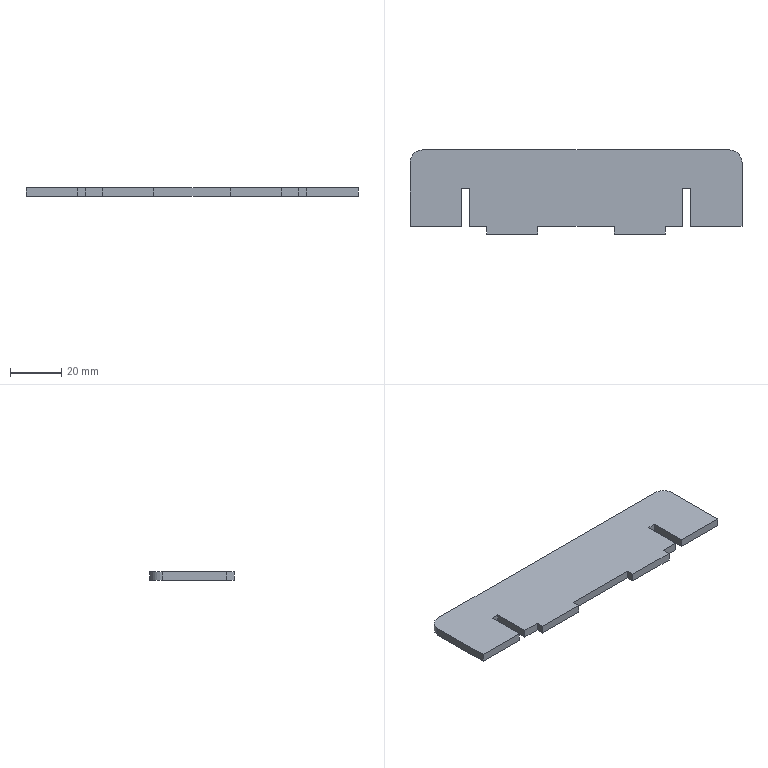Part | SolidWorks | features FlatPattern 1, SMBaseFlange 1, SheetMetal 1 | 1 solid | 24 faces | box 130 x 33 x 3.2 mm | volume 12522 mm3 | plane 22 | cylinder 2 | commonest cylinder face diameters 10 x2
STEP:
#1=CARTESIAN_POINT('',(51.242,-108.501,0.));
#2=VERTEX_POINT('',#1);
#3=CARTESIAN_POINT('',(51.242,-83.501,0.));
#4=VERTEX_POINT('',#3);
#5=CARTESIAN_POINT('',(51.242,-108.501,0.));
#6=DIRECTION('',(0.,1.,0.));
#7=VECTOR('',#6,1000.);
#8=LINE('',#5,#7);
#9=EDGE_CURVE('',#2,#4,#8,.T.);
#10=ORIENTED_EDGE('',*,*,#9,.F.);
#11=CARTESIAN_POINT('',(51.242,-108.501,-3.2));
#12=VERTEX_POINT('',#11);
#13=CARTESIAN_POINT('',(51.242,-108.501,-3.2));
#14=DIRECTION('',(0.,0.,1.));
#15=VECTOR('',#14,1000.);
#16=LINE('',#13,#15);
#17=EDGE_CURVE('',#12,#2,#16,.T.);
#18=ORIENTED_EDGE('',*,*,#17,.F.);
#19=CARTESIAN_POINT('',(51.242,-83.501,-3.2));
#20=VERTEX_POINT('',#19);
#21=CARTESIAN_POINT('',(51.242,-108.501,-3.2));
#22=DIRECTION('',(0.,1.,0.));
#23=VECTOR('',#22,1000.);
#24=LINE('',#21,#23);
#25=EDGE_CURVE('',#12,#20,#24,.T.);
#26=ORIENTED_EDGE('',*,*,#25,.T.);
#27=CARTESIAN_POINT('',(51.242,-83.501,-3.2));
#28=DIRECTION('',(0.,0.,1.));
#29=VECTOR('',#28,1000.);
#30=LINE('',#27,#29);
#31=EDGE_CURVE('',#20,#4,#30,.T.);
#32=ORIENTED_EDGE('',*,*,#31,.T.);
#33=EDGE_LOOP('',(#10,#18,#26,#32));
#34=FACE_OUTER_BOUND('',#33,.T.);
#35=CARTESIAN_POINT('',(51.242,-108.501,-3.2));
#36=DIRECTION('',(1.,0.,0.));
#37=DIRECTION('',(0.,0.,-1.));
#38=AXIS2_PLACEMENT_3D('',#35,#36,#37);
#39=PLANE('',#38);
#40=ADVANCED_FACE('',(#34),#39,.T.);
#41=CARTESIAN_POINT('',(31.242,-108.501,0.));
#42=VERTEX_POINT('',#41);
#43=CARTESIAN_POINT('',(51.242,-108.501,0.));
#44=DIRECTION('',(1.,0.,0.));
#45=VECTOR('',#44,1000.);
#46=LINE('',#43,#45);
#47=EDGE_CURVE('',#42,#2,#46,.T.);
#48=ORIENTED_EDGE('',*,*,#47,.F.);
#49=CARTESIAN_POINT('',(31.242,-108.501,-3.2));
#50=VERTEX_POINT('',#49);
#51=CARTESIAN_POINT('',(31.242,-108.501,-3.2));
#52=DIRECTION('',(0.,0.,1.));
#53=VECTOR('',#52,1000.);
#54=LINE('',#51,#53);
#55=EDGE_CURVE('',#50,#42,#54,.T.);
#56=ORIENTED_EDGE('',*,*,#55,.F.);
#57=CARTESIAN_POINT('',(51.242,-108.501,-3.2));
#58=DIRECTION('',(1.,0.,0.));
#59=VECTOR('',#58,1000.);
#60=LINE('',#57,#59);
#61=EDGE_CURVE('',#50,#12,#60,.T.);
#62=ORIENTED_EDGE('',*,*,#61,.T.);
#63=ORIENTED_EDGE('',*,*,#17,.T.);
#64=EDGE_LOOP('',(#48,#56,#62,#63));
#65=FACE_OUTER_BOUND('',#64,.T.);
#66=CARTESIAN_POINT('',(51.242,-108.501,-3.2));
#67=DIRECTION('',(0.,-1.,0.));
#68=DIRECTION('',(0.,0.,-1.));
#69=AXIS2_PLACEMENT_3D('',#66,#67,#68);
#70=PLANE('',#69);
#71=ADVANCED_FACE('',(#65),#70,.T.);
#72=CARTESIAN_POINT('',(31.242,-93.501,0.));
#73=VERTEX_POINT('',#72);
#74=CARTESIAN_POINT('',(31.242,-93.501,0.));
#75=DIRECTION('',(0.,-1.,0.));
#76=VECTOR('',#75,1000.);
#77=LINE('',#74,#76);
#78=EDGE_CURVE('',#73,#42,#77,.T.);
#79=ORIENTED_EDGE('',*,*,#78,.F.);
#80=CARTESIAN_POINT('',(31.242,-93.501,-3.2));
#81=VERTEX_POINT('',#80);
#82=CARTESIAN_POINT('',(31.242,-93.501,-3.2));
#83=DIRECTION('',(0.,0.,1.));
#84=VECTOR('',#83,1000.);
#85=LINE('',#82,#84);
#86=EDGE_CURVE('',#81,#73,#85,.T.);
#87=ORIENTED_EDGE('',*,*,#86,.F.);
#88=CARTESIAN_POINT('',(31.242,-93.501,-3.2));
#89=DIRECTION('',(0.,-1.,0.));
#90=VECTOR('',#89,1000.);
#91=LINE('',#88,#90);
#92=EDGE_CURVE('',#81,#50,#91,.T.);
#93=ORIENTED_EDGE('',*,*,#92,.T.);
#94=ORIENTED_EDGE('',*,*,#55,.T.);
#95=EDGE_LOOP('',(#79,#87,#93,#94));
#96=FACE_OUTER_BOUND('',#95,.T.);
#97=CARTESIAN_POINT('',(31.242,-93.501,-3.2));
#98=DIRECTION('',(-1.,0.,0.));
#99=DIRECTION('',(0.,0.,1.));
#100=AXIS2_PLACEMENT_3D('',#97,#98,#99);
#101=PLANE('',#100);
#102=ADVANCED_FACE('',(#96),#101,.T.);
#103=CARTESIAN_POINT('',(28.042,-93.501,0.));
#104=VERTEX_POINT('',#103);
#105=CARTESIAN_POINT('',(31.242,-93.501,0.));
#106=DIRECTION('',(1.,0.,0.));
#107=VECTOR('',#106,1000.);
#108=LINE('',#105,#107);
#109=EDGE_CURVE('',#104,#73,#108,.T.);
#110=ORIENTED_EDGE('',*,*,#109,.F.);
#111=CARTESIAN_POINT('',(28.042,-93.501,-3.2));
#112=VERTEX_POINT('',#111);
#113=CARTESIAN_POINT('',(28.042,-93.501,-3.2));
#114=DIRECTION('',(0.,0.,1.));
#115=VECTOR('',#114,1000.);
#116=LINE('',#113,#115);
#117=EDGE_CURVE('',#112,#104,#116,.T.);
#118=ORIENTED_EDGE('',*,*,#117,.F.);
#119=CARTESIAN_POINT('',(31.242,-93.501,-3.2));
#120=DIRECTION('',(1.,0.,0.));
#121=VECTOR('',#120,1000.);
#122=LINE('',#119,#121);
#123=EDGE_CURVE('',#112,#81,#122,.T.);
#124=ORIENTED_EDGE('',*,*,#123,.T.);
#125=ORIENTED_EDGE('',*,*,#86,.T.);
#126=EDGE_LOOP('',(#110,#118,#124,#125));
#127=FACE_OUTER_BOUND('',#126,.T.);
#128=CARTESIAN_POINT('',(31.242,-93.501,-3.2));
#129=DIRECTION('',(0.,-1.,0.));
#130=DIRECTION('',(0.,0.,-1.));
#131=AXIS2_PLACEMENT_3D('',#128,#129,#130);
#132=PLANE('',#131);
#133=ADVANCED_FACE('',(#127),#132,.T.);
#134=CARTESIAN_POINT('',(28.042,-108.501,0.));
#135=VERTEX_POINT('',#134);
#136=CARTESIAN_POINT('',(28.042,-93.501,0.));
#137=DIRECTION('',(0.,1.,0.));
#138=VECTOR('',#137,1000.);
#139=LINE('',#136,#138);
#140=EDGE_CURVE('',#135,#104,#139,.T.);
#141=ORIENTED_EDGE('',*,*,#140,.F.);
#142=CARTESIAN_POINT('',(28.042,-108.501,-3.2));
#143=VERTEX_POINT('',#142);
#144=CARTESIAN_POINT('',(28.042,-108.501,-3.2));
#145=DIRECTION('',(0.,0.,1.));
#146=VECTOR('',#145,1000.);
#147=LINE('',#144,#146);
#148=EDGE_CURVE('',#143,#135,#147,.T.);
#149=ORIENTED_EDGE('',*,*,#148,.F.);
#150=CARTESIAN_POINT('',(28.042,-93.501,-3.2));
#151=DIRECTION('',(0.,1.,0.));
#152=VECTOR('',#151,1000.);
#153=LINE('',#150,#152);
#154=EDGE_CURVE('',#143,#112,#153,.T.);
#155=ORIENTED_EDGE('',*,*,#154,.T.);
#156=ORIENTED_EDGE('',*,*,#117,.T.);
#157=EDGE_LOOP('',(#141,#149,#155,#156));
#158=FACE_OUTER_BOUND('',#157,.T.);
#159=CARTESIAN_POINT('',(28.042,-93.501,-3.2));
#160=DIRECTION('',(1.,0.,0.));
#161=DIRECTION('',(0.,0.,-1.));
#162=AXIS2_PLACEMENT_3D('',#159,#160,#161);
#163=PLANE('',#162);
#164=ADVANCED_FACE('',(#158),#163,.T.);
#165=CARTESIAN_POINT('',(21.242,-108.501,0.));
#166=VERTEX_POINT('',#165);
#167=CARTESIAN_POINT('',(28.042,-108.501,0.));
#168=DIRECTION('',(1.,0.,0.));
#169=VECTOR('',#168,1000.);
#170=LINE('',#167,#169);
#171=EDGE_CURVE('',#166,#135,#170,.T.);
#172=ORIENTED_EDGE('',*,*,#171,.F.);
#173=CARTESIAN_POINT('',(21.242,-108.501,-3.2));
#174=VERTEX_POINT('',#173);
#175=CARTESIAN_POINT('',(21.242,-108.501,-3.2));
#176=DIRECTION('',(0.,0.,1.));
#177=VECTOR('',#176,1000.);
#178=LINE('',#175,#177);
#179=EDGE_CURVE('',#174,#166,#178,.T.);
#180=ORIENTED_EDGE('',*,*,#179,.F.);
#181=CARTESIAN_POINT('',(28.042,-108.501,-3.2));
#182=DIRECTION('',(1.,0.,0.));
#183=VECTOR('',#182,1000.);
#184=LINE('',#181,#183);
#185=EDGE_CURVE('',#174,#143,#184,.T.);
#186=ORIENTED_EDGE('',*,*,#185,.T.);
#187=ORIENTED_EDGE('',*,*,#148,.T.);
#188=EDGE_LOOP('',(#172,#180,#186,#187));
#189=FACE_OUTER_BOUND('',#188,.T.);
#190=CARTESIAN_POINT('',(28.042,-108.501,-3.2));
#191=DIRECTION('',(0.,-1.,0.));
#192=DIRECTION('',(0.,0.,-1.));
#193=AXIS2_PLACEMENT_3D('',#190,#191,#192);
#194=PLANE('',#193);
#195=ADVANCED_FACE('',(#189),#194,.T.);
#196=CARTESIAN_POINT('',(21.242,-111.501,0.));
#197=VERTEX_POINT('',#196);
#198=CARTESIAN_POINT('',(21.242,-108.501,0.));
#199=DIRECTION('',(0.,1.,0.));
#200=VECTOR('',#199,1000.);
#201=LINE('',#198,#200);
#202=EDGE_CURVE('',#197,#166,#201,.T.);
#203=ORIENTED_EDGE('',*,*,#202,.F.);
#204=CARTESIAN_POINT('',(21.242,-111.501,-3.2));
#205=VERTEX_POINT('',#204);
#206=CARTESIAN_POINT('',(21.242,-111.501,-3.2));
#207=DIRECTION('',(0.,0.,1.));
#208=VECTOR('',#207,1000.);
#209=LINE('',#206,#208);
#210=EDGE_CURVE('',#205,#197,#209,.T.);
#211=ORIENTED_EDGE('',*,*,#210,.F.);
#212=CARTESIAN_POINT('',(21.242,-108.501,-3.2));
#213=DIRECTION('',(0.,1.,0.));
#214=VECTOR('',#213,1000.);
#215=LINE('',#212,#214);
#216=EDGE_CURVE('',#205,#174,#215,.T.);
#217=ORIENTED_EDGE('',*,*,#216,.T.);
#218=ORIENTED_EDGE('',*,*,#179,.T.);
#219=EDGE_LOOP('',(#203,#211,#217,#218));
#220=FACE_OUTER_BOUND('',#219,.T.);
#221=CARTESIAN_POINT('',(21.242,-108.501,-3.2));
#222=DIRECTION('',(1.,0.,0.));
#223=DIRECTION('',(0.,0.,-1.));
#224=AXIS2_PLACEMENT_3D('',#221,#222,#223);
#225=PLANE('',#224);
#226=ADVANCED_FACE('',(#220),#225,.T.);
#227=CARTESIAN_POINT('',(1.242,-111.501,0.));
#228=VERTEX_POINT('',#227);
#229=CARTESIAN_POINT('',(21.242,-111.501,0.));
#230=DIRECTION('',(1.,0.,0.));
#231=VECTOR('',#230,1000.);
#232=LINE('',#229,#231);
#233=EDGE_CURVE('',#228,#197,#232,.T.);
#234=ORIENTED_EDGE('',*,*,#233,.F.);
#235=CARTESIAN_POINT('',(1.242,-111.501,-3.2));
#236=VERTEX_POINT('',#235);
#237=CARTESIAN_POINT('',(1.242,-111.501,-3.2));
#238=DIRECTION('',(0.,0.,1.));
#239=VECTOR('',#238,1000.);
#240=LINE('',#237,#239);
#241=EDGE_CURVE('',#236,#228,#240,.T.);
#242=ORIENTED_EDGE('',*,*,#241,.F.);
#243=CARTESIAN_POINT('',(21.242,-111.501,-3.2));
#244=DIRECTION('',(1.,0.,0.));
#245=VECTOR('',#244,1000.);
#246=LINE('',#243,#245);
#247=EDGE_CURVE('',#236,#205,#246,.T.);
#248=ORIENTED_EDGE('',*,*,#247,.T.);
#249=ORIENTED_EDGE('',*,*,#210,.T.);
#250=EDGE_LOOP('',(#234,#242,#248,#249));
#251=FACE_OUTER_BOUND('',#250,.T.);
#252=CARTESIAN_POINT('',(21.242,-111.501,-3.2));
#253=DIRECTION('',(0.,-1.,0.));
#254=DIRECTION('',(0.,0.,-1.));
#255=AXIS2_PLACEMENT_3D('',#252,#253,#254);
#256=PLANE('',#255);
#257=ADVANCED_FACE('',(#251),#256,.T.);
#258=CARTESIAN_POINT('',(1.242,-108.501,0.));
#259=VERTEX_POINT('',#258);
#260=CARTESIAN_POINT('',(1.242,-111.501,0.));
#261=DIRECTION('',(0.,-1.,0.));
#262=VECTOR('',#261,1000.);
#263=LINE('',#260,#262);
#264=EDGE_CURVE('',#259,#228,#263,.T.);
#265=ORIENTED_EDGE('',*,*,#264,.F.);
#266=CARTESIAN_POINT('',(1.242,-108.501,-3.2));
#267=VERTEX_POINT('',#266);
#268=CARTESIAN_POINT('',(1.242,-108.501,-3.2));
#269=DIRECTION('',(0.,0.,1.));
#270=VECTOR('',#269,1000.);
#271=LINE('',#268,#270);
#272=EDGE_CURVE('',#267,#259,#271,.T.);
#273=ORIENTED_EDGE('',*,*,#272,.F.);
#274=CARTESIAN_POINT('',(1.242,-111.501,-3.2));
#275=DIRECTION('',(0.,-1.,0.));
#276=VECTOR('',#275,1000.);
#277=LINE('',#274,#276);
#278=EDGE_CURVE('',#267,#236,#277,.T.);
#279=ORIENTED_EDGE('',*,*,#278,.T.);
#280=ORIENTED_EDGE('',*,*,#241,.T.);
#281=EDGE_LOOP('',(#265,#273,#279,#280));
#282=FACE_OUTER_BOUND('',#281,.T.);
#283=CARTESIAN_POINT('',(1.242,-111.501,-3.2));
#284=DIRECTION('',(-1.,0.,0.));
#285=DIRECTION('',(0.,0.,1.));
#286=AXIS2_PLACEMENT_3D('',#283,#284,#285);
#287=PLANE('',#286);
#288=ADVANCED_FACE('',(#282),#287,.T.);
#289=CARTESIAN_POINT('',(-28.758,-108.501,0.));
#290=VERTEX_POINT('',#289);
#291=CARTESIAN_POINT('',(1.242,-108.501,0.));
#292=DIRECTION('',(1.,0.,0.));
#293=VECTOR('',#292,1000.);
#294=LINE('',#291,#293);
#295=EDGE_CURVE('',#290,#259,#294,.T.);
#296=ORIENTED_EDGE('',*,*,#295,.F.);
#297=CARTESIAN_POINT('',(-28.758,-108.501,-3.2));
#298=VERTEX_POINT('',#297);
#299=CARTESIAN_POINT('',(-28.758,-108.501,-3.2));
#300=DIRECTION('',(0.,0.,1.));
#301=VECTOR('',#300,1000.);
#302=LINE('',#299,#301);
#303=EDGE_CURVE('',#298,#290,#302,.T.);
#304=ORIENTED_EDGE('',*,*,#303,.F.);
#305=CARTESIAN_POINT('',(1.242,-108.501,-3.2));
#306=DIRECTION('',(1.,0.,0.));
#307=VECTOR('',#306,1000.);
#308=LINE('',#305,#307);
#309=EDGE_CURVE('',#298,#267,#308,.T.);
#310=ORIENTED_EDGE('',*,*,#309,.T.);
#311=ORIENTED_EDGE('',*,*,#272,.T.);
#312=EDGE_LOOP('',(#296,#304,#310,#311));
#313=FACE_OUTER_BOUND('',#312,.T.);
#314=CARTESIAN_POINT('',(1.242,-108.501,-3.2));
#315=DIRECTION('',(0.,-1.,0.));
#316=DIRECTION('',(0.,0.,-1.));
#317=AXIS2_PLACEMENT_3D('',#314,#315,#316);
#318=PLANE('',#317);
#319=ADVANCED_FACE('',(#313),#318,.T.);
#320=CARTESIAN_POINT('',(-28.758,-111.501,0.));
#321=VERTEX_POINT('',#320);
#322=CARTESIAN_POINT('',(-28.758,-111.501,0.));
#323=DIRECTION('',(0.,1.,0.));
#324=VECTOR('',#323,1000.);
#325=LINE('',#322,#324);
#326=EDGE_CURVE('',#321,#290,#325,.T.);
#327=ORIENTED_EDGE('',*,*,#326,.F.);
#328=CARTESIAN_POINT('',(-28.758,-111.501,-3.2));
#329=VERTEX_POINT('',#328);
#330=CARTESIAN_POINT('',(-28.758,-111.501,-3.2));
#331=DIRECTION('',(0.,0.,1.));
#332=VECTOR('',#331,1000.);
#333=LINE('',#330,#332);
#334=EDGE_CURVE('',#329,#321,#333,.T.);
#335=ORIENTED_EDGE('',*,*,#334,.F.);
#336=CARTESIAN_POINT('',(-28.758,-111.501,-3.2));
#337=DIRECTION('',(0.,1.,0.));
#338=VECTOR('',#337,1000.);
#339=LINE('',#336,#338);
#340=EDGE_CURVE('',#329,#298,#339,.T.);
#341=ORIENTED_EDGE('',*,*,#340,.T.);
#342=ORIENTED_EDGE('',*,*,#303,.T.);
#343=EDGE_LOOP('',(#327,#335,#341,#342));
#344=FACE_OUTER_BOUND('',#343,.T.);
#345=CARTESIAN_POINT('',(-28.758,-111.501,-3.2));
#346=DIRECTION('',(1.,0.,0.));
#347=DIRECTION('',(0.,0.,-1.));
#348=AXIS2_PLACEMENT_3D('',#345,#346,#347);
#349=PLANE('',#348);
#350=ADVANCED_FACE('',(#344),#349,.T.);
#351=CARTESIAN_POINT('',(-48.758,-111.501,0.));
#352=VERTEX_POINT('',#351);
#353=CARTESIAN_POINT('',(-48.758,-111.501,0.));
#354=DIRECTION('',(1.,0.,0.));
#355=VECTOR('',#354,1000.);
#356=LINE('',#353,#355);
#357=EDGE_CURVE('',#352,#321,#356,.T.);
#358=ORIENTED_EDGE('',*,*,#357,.F.);
#359=CARTESIAN_POINT('',(-48.758,-111.501,-3.2));
#360=VERTEX_POINT('',#359);
#361=CARTESIAN_POINT('',(-48.758,-111.501,-3.2));
#362=DIRECTION('',(0.,0.,1.));
#363=VECTOR('',#362,1000.);
#364=LINE('',#361,#363);
#365=EDGE_CURVE('',#360,#352,#364,.T.);
#366=ORIENTED_EDGE('',*,*,#365,.F.);
#367=CARTESIAN_POINT('',(-48.758,-111.501,-3.2));
#368=DIRECTION('',(1.,0.,0.));
#369=VECTOR('',#368,1000.);
#370=LINE('',#367,#369);
#371=EDGE_CURVE('',#360,#329,#370,.T.);
#372=ORIENTED_EDGE('',*,*,#371,.T.);
#373=ORIENTED_EDGE('',*,*,#334,.T.);
#374=EDGE_LOOP('',(#358,#366,#372,#373));
#375=FACE_OUTER_BOUND('',#374,.T.);
#376=CARTESIAN_POINT('',(-48.758,-111.501,-3.2));
#377=DIRECTION('',(0.,-1.,0.));
#378=DIRECTION('',(0.,0.,-1.));
#379=AXIS2_PLACEMENT_3D('',#376,#377,#378);
#380=PLANE('',#379);
#381=ADVANCED_FACE('',(#375),#380,.T.);
#382=CARTESIAN_POINT('',(-48.758,-108.501,0.));
#383=VERTEX_POINT('',#382);
#384=CARTESIAN_POINT('',(-48.758,-108.501,0.));
#385=DIRECTION('',(0.,-1.,0.));
#386=VECTOR('',#385,1000.);
#387=LINE('',#384,#386);
#388=EDGE_CURVE('',#383,#352,#387,.T.);
#389=ORIENTED_EDGE('',*,*,#388,.F.);
#390=CARTESIAN_POINT('',(-48.758,-108.501,-3.2));
#391=VERTEX_POINT('',#390);
#392=CARTESIAN_POINT('',(-48.758,-108.501,-3.2));
#393=DIRECTION('',(0.,0.,1.));
#394=VECTOR('',#393,1000.);
#395=LINE('',#392,#394);
#396=EDGE_CURVE('',#391,#383,#395,.T.);
#397=ORIENTED_EDGE('',*,*,#396,.F.);
#398=CARTESIAN_POINT('',(-48.758,-108.501,-3.2));
#399=DIRECTION('',(0.,-1.,0.));
#400=VECTOR('',#399,1000.);
#401=LINE('',#398,#400);
#402=EDGE_CURVE('',#391,#360,#401,.T.);
#403=ORIENTED_EDGE('',*,*,#402,.T.);
#404=ORIENTED_EDGE('',*,*,#365,.T.);
#405=EDGE_LOOP('',(#389,#397,#403,#404));
#406=FACE_OUTER_BOUND('',#405,.T.);
#407=CARTESIAN_POINT('',(-48.758,-108.501,-3.2));
#408=DIRECTION('',(-1.,0.,0.));
#409=DIRECTION('',(0.,0.,1.));
#410=AXIS2_PLACEMENT_3D('',#407,#408,#409);
#411=PLANE('',#410);
#412=ADVANCED_FACE('',(#406),#411,.T.);
#413=CARTESIAN_POINT('',(-55.558,-108.501,0.));
#414=VERTEX_POINT('',#413);
#415=CARTESIAN_POINT('',(-48.758,-108.501,0.));
#416=DIRECTION('',(1.,0.,0.));
#417=VECTOR('',#416,1000.);
#418=LINE('',#415,#417);
#419=EDGE_CURVE('',#414,#383,#418,.T.);
#420=ORIENTED_EDGE('',*,*,#419,.F.);
#421=CARTESIAN_POINT('',(-55.558,-108.501,-3.2));
#422=VERTEX_POINT('',#421);
#423=CARTESIAN_POINT('',(-55.558,-108.501,-3.2));
#424=DIRECTION('',(0.,0.,1.));
#425=VECTOR('',#424,1000.);
#426=LINE('',#423,#425);
#427=EDGE_CURVE('',#422,#414,#426,.T.);
#428=ORIENTED_EDGE('',*,*,#427,.F.);
#429=CARTESIAN_POINT('',(-48.758,-108.501,-3.2));
#430=DIRECTION('',(1.,0.,0.));
#431=VECTOR('',#430,1000.);
#432=LINE('',#429,#431);
#433=EDGE_CURVE('',#422,#391,#432,.T.);
#434=ORIENTED_EDGE('',*,*,#433,.T.);
#435=ORIENTED_EDGE('',*,*,#396,.T.);
#436=EDGE_LOOP('',(#420,#428,#434,#435));
#437=FACE_OUTER_BOUND('',#436,.T.);
#438=CARTESIAN_POINT('',(-48.758,-108.501,-3.2));
#439=DIRECTION('',(0.,-1.,0.));
#440=DIRECTION('',(1.,0.,0.));
#441=AXIS2_PLACEMENT_3D('',#438,#439,#440);
#442=PLANE('',#441);
#443=ADVANCED_FACE('',(#437),#442,.T.);
#444=CARTESIAN_POINT('',(-55.558,-93.501,0.));
#445=VERTEX_POINT('',#444);
#446=CARTESIAN_POINT('',(-55.558,-108.501,0.));
#447=DIRECTION('',(0.,-1.,0.));
#448=VECTOR('',#447,1000.);
#449=LINE('',#446,#448);
#450=EDGE_CURVE('',#445,#414,#449,.T.);
#451=ORIENTED_EDGE('',*,*,#450,.F.);
#452=CARTESIAN_POINT('',(-55.558,-93.501,-3.2));
#453=VERTEX_POINT('',#452);
#454=CARTESIAN_POINT('',(-55.558,-93.501,-3.2));
#455=DIRECTION('',(0.,0.,1.));
#456=VECTOR('',#455,1000.);
#457=LINE('',#454,#456);
#458=EDGE_CURVE('',#453,#445,#457,.T.);
#459=ORIENTED_EDGE('',*,*,#458,.F.);
#460=CARTESIAN_POINT('',(-55.558,-108.501,-3.2));
#461=DIRECTION('',(0.,-1.,0.));
#462=VECTOR('',#461,1000.);
#463=LINE('',#460,#462);
#464=EDGE_CURVE('',#453,#422,#463,.T.);
#465=ORIENTED_EDGE('',*,*,#464,.T.);
#466=ORIENTED_EDGE('',*,*,#427,.T.);
#467=EDGE_LOOP('',(#451,#459,#465,#466));
#468=FACE_OUTER_BOUND('',#467,.T.);
#469=CARTESIAN_POINT('',(-55.558,-108.501,-3.2));
#470=DIRECTION('',(-1.,0.,0.));
#471=DIRECTION('',(0.,0.,1.));
#472=AXIS2_PLACEMENT_3D('',#469,#470,#471);
#473=PLANE('',#472);
#474=ADVANCED_FACE('',(#468),#473,.T.);
#475=CARTESIAN_POINT('',(-58.758,-93.501,0.));
#476=VERTEX_POINT('',#475);
#477=CARTESIAN_POINT('',(-55.558,-93.501,0.));
#478=DIRECTION('',(1.,0.,0.));
#479=VECTOR('',#478,1000.);
#480=LINE('',#477,#479);
#481=EDGE_CURVE('',#476,#445,#480,.T.);
#482=ORIENTED_EDGE('',*,*,#481,.F.);
#483=CARTESIAN_POINT('',(-58.758,-93.501,-3.2));
#484=VERTEX_POINT('',#483);
#485=CARTESIAN_POINT('',(-58.758,-93.501,-3.2));
#486=DIRECTION('',(0.,0.,1.));
#487=VECTOR('',#486,1000.);
#488=LINE('',#485,#487);
#489=EDGE_CURVE('',#484,#476,#488,.T.);
#490=ORIENTED_EDGE('',*,*,#489,.F.);
#491=CARTESIAN_POINT('',(-55.558,-93.501,-3.2));
#492=DIRECTION('',(1.,0.,0.));
#493=VECTOR('',#492,1000.);
#494=LINE('',#491,#493);
#495=EDGE_CURVE('',#484,#453,#494,.T.);
#496=ORIENTED_EDGE('',*,*,#495,.T.);
#497=ORIENTED_EDGE('',*,*,#458,.T.);
#498=EDGE_LOOP('',(#482,#490,#496,#497));
#499=FACE_OUTER_BOUND('',#498,.T.);
#500=CARTESIAN_POINT('',(-55.558,-93.501,-3.2));
#501=DIRECTION('',(0.,-1.,0.));
#502=DIRECTION('',(0.,0.,-1.));
#503=AXIS2_PLACEMENT_3D('',#500,#501,#502);
#504=PLANE('',#503);
#505=ADVANCED_FACE('',(#499),#504,.T.);
#506=CARTESIAN_POINT('',(-58.758,-108.501,0.));
#507=VERTEX_POINT('',#506);
#508=CARTESIAN_POINT('',(-58.758,-93.501,0.));
#509=DIRECTION('',(0.,1.,0.));
#510=VECTOR('',#509,1000.);
#511=LINE('',#508,#510);
#512=EDGE_CURVE('',#507,#476,#511,.T.);
#513=ORIENTED_EDGE('',*,*,#512,.F.);
#514=CARTESIAN_POINT('',(-58.758,-108.501,-3.2));
#515=VERTEX_POINT('',#514);
#516=CARTESIAN_POINT('',(-58.758,-108.501,-3.2));
#517=DIRECTION('',(0.,0.,1.));
#518=VECTOR('',#517,1000.);
#519=LINE('',#516,#518);
#520=EDGE_CURVE('',#515,#507,#519,.T.);
#521=ORIENTED_EDGE('',*,*,#520,.F.);
#522=CARTESIAN_POINT('',(-58.758,-93.501,-3.2));
#523=DIRECTION('',(0.,1.,0.));
#524=VECTOR('',#523,1000.);
#525=LINE('',#522,#524);
#526=EDGE_CURVE('',#515,#484,#525,.T.);
#527=ORIENTED_EDGE('',*,*,#526,.T.);
#528=ORIENTED_EDGE('',*,*,#489,.T.);
#529=EDGE_LOOP('',(#513,#521,#527,#528));
#530=FACE_OUTER_BOUND('',#529,.T.);
#531=CARTESIAN_POINT('',(-58.758,-93.501,-3.2));
#532=DIRECTION('',(1.,0.,0.));
#533=DIRECTION('',(0.,0.,-1.));
#534=AXIS2_PLACEMENT_3D('',#531,#532,#533);
#535=PLANE('',#534);
#536=ADVANCED_FACE('',(#530),#535,.T.);
#537=CARTESIAN_POINT('',(-78.758,-108.501,0.));
#538=VERTEX_POINT('',#537);
#539=CARTESIAN_POINT('',(-58.758,-108.501,0.));
#540=DIRECTION('',(1.,0.,0.));
#541=VECTOR('',#540,1000.);
#542=LINE('',#539,#541);
#543=EDGE_CURVE('',#538,#507,#542,.T.);
#544=ORIENTED_EDGE('',*,*,#543,.F.);
#545=CARTESIAN_POINT('',(-78.758,-108.501,-3.2));
#546=VERTEX_POINT('',#545);
#547=CARTESIAN_POINT('',(-78.758,-108.501,-3.2));
#548=DIRECTION('',(0.,0.,1.));
#549=VECTOR('',#548,1000.);
#550=LINE('',#547,#549);
#551=EDGE_CURVE('',#546,#538,#550,.T.);
#552=ORIENTED_EDGE('',*,*,#551,.F.);
#553=CARTESIAN_POINT('',(-58.758,-108.501,-3.2));
#554=DIRECTION('',(1.,0.,0.));
#555=VECTOR('',#554,1000.);
#556=LINE('',#553,#555);
#557=EDGE_CURVE('',#546,#515,#556,.T.);
#558=ORIENTED_EDGE('',*,*,#557,.T.);
#559=ORIENTED_EDGE('',*,*,#520,.T.);
#560=EDGE_LOOP('',(#544,#552,#558,#559));
#561=FACE_OUTER_BOUND('',#560,.T.);
#562=CARTESIAN_POINT('',(-58.758,-108.501,-3.2));
#563=DIRECTION('',(0.,-1.,0.));
#564=DIRECTION('',(0.,0.,-1.));
#565=AXIS2_PLACEMENT_3D('',#562,#563,#564);
#566=PLANE('',#565);
#567=ADVANCED_FACE('',(#561),#566,.T.);
#568=CARTESIAN_POINT('',(-78.758,-83.501,0.));
#569=VERTEX_POINT('',#568);
#570=CARTESIAN_POINT('',(-78.758,-108.501,0.));
#571=DIRECTION('',(0.,-1.,0.));
#572=VECTOR('',#571,1000.);
#573=LINE('',#570,#572);
#574=EDGE_CURVE('',#569,#538,#573,.T.);
#575=ORIENTED_EDGE('',*,*,#574,.F.);
#576=CARTESIAN_POINT('',(-78.758,-83.501,-3.2));
#577=VERTEX_POINT('',#576);
#578=CARTESIAN_POINT('',(-78.758,-83.501,-3.2));
#579=DIRECTION('',(0.,0.,1.));
#580=VECTOR('',#579,1000.);
#581=LINE('',#578,#580);
#582=EDGE_CURVE('',#577,#569,#581,.T.);
#583=ORIENTED_EDGE('',*,*,#582,.F.);
#584=CARTESIAN_POINT('',(-78.758,-108.501,-3.2));
#585=DIRECTION('',(0.,-1.,0.));
#586=VECTOR('',#585,1000.);
#587=LINE('',#584,#586);
#588=EDGE_CURVE('',#577,#546,#587,.T.);
#589=ORIENTED_EDGE('',*,*,#588,.T.);
#590=ORIENTED_EDGE('',*,*,#551,.T.);
#591=EDGE_LOOP('',(#575,#583,#589,#590));
#592=FACE_OUTER_BOUND('',#591,.T.);
#593=CARTESIAN_POINT('',(-78.758,-108.501,-3.2));
#594=DIRECTION('',(-1.,0.,0.));
#595=DIRECTION('',(0.,0.,1.));
#596=AXIS2_PLACEMENT_3D('',#593,#594,#595);
#597=PLANE('',#596);
#598=ADVANCED_FACE('',(#592),#597,.T.);
#599=CARTESIAN_POINT('',(-73.758,-78.501,0.));
#600=VERTEX_POINT('',#599);
#601=CARTESIAN_POINT('',(-73.758,-83.501,0.));
#602=DIRECTION('',(0.,0.,1.));
#603=DIRECTION('',(1.,0.,0.));
#604=AXIS2_PLACEMENT_3D('',#601,#602,#603);
#605=CIRCLE('',#604,5.);
#606=EDGE_CURVE('',#600,#569,#605,.T.);
#607=ORIENTED_EDGE('',*,*,#606,.F.);
#608=CARTESIAN_POINT('',(-73.758,-78.501,-3.2));
#609=VERTEX_POINT('',#608);
#610=CARTESIAN_POINT('',(-73.758,-78.501,-3.2));
#611=DIRECTION('',(0.,0.,1.));
#612=VECTOR('',#611,1000.);
#613=LINE('',#610,#612);
#614=EDGE_CURVE('',#609,#600,#613,.T.);
#615=ORIENTED_EDGE('',*,*,#614,.F.);
#616=CARTESIAN_POINT('',(-73.758,-83.501,-3.2));
#617=DIRECTION('',(0.,0.,1.));
#618=DIRECTION('',(1.,0.,0.));
#619=AXIS2_PLACEMENT_3D('',#616,#617,#618);
#620=CIRCLE('',#619,5.);
#621=EDGE_CURVE('',#609,#577,#620,.T.);
#622=ORIENTED_EDGE('',*,*,#621,.T.);
#623=ORIENTED_EDGE('',*,*,#582,.T.);
#624=EDGE_LOOP('',(#607,#615,#622,#623));
#625=FACE_OUTER_BOUND('',#624,.T.);
#626=CARTESIAN_POINT('',(-73.758,-83.501,-3.2));
#627=DIRECTION('',(0.,0.,1.));
#628=DIRECTION('',(1.,0.,0.));
#629=AXIS2_PLACEMENT_3D('',#626,#627,#628);
#630=CYLINDRICAL_SURFACE('',#629,5.);
#631=ADVANCED_FACE('',(#625),#630,.T.);
#632=CARTESIAN_POINT('',(46.242,-78.501,0.));
#633=VERTEX_POINT('',#632);
#634=CARTESIAN_POINT('',(46.242,-78.501,0.));
#635=DIRECTION('',(-1.,0.,0.));
#636=VECTOR('',#635,1000.);
#637=LINE('',#634,#636);
#638=EDGE_CURVE('',#633,#600,#637,.T.);
#639=ORIENTED_EDGE('',*,*,#638,.F.);
#640=CARTESIAN_POINT('',(46.242,-78.501,-3.2));
#641=VERTEX_POINT('',#640);
#642=CARTESIAN_POINT('',(46.242,-78.501,-3.2));
#643=DIRECTION('',(0.,0.,1.));
#644=VECTOR('',#643,1000.);
#645=LINE('',#642,#644);
#646=EDGE_CURVE('',#641,#633,#645,.T.);
#647=ORIENTED_EDGE('',*,*,#646,.F.);
#648=CARTESIAN_POINT('',(46.242,-78.501,-3.2));
#649=DIRECTION('',(-1.,0.,0.));
#650=VECTOR('',#649,1000.);
#651=LINE('',#648,#650);
#652=EDGE_CURVE('',#641,#609,#651,.T.);
#653=ORIENTED_EDGE('',*,*,#652,.T.);
#654=ORIENTED_EDGE('',*,*,#614,.T.);
#655=EDGE_LOOP('',(#639,#647,#653,#654));
#656=FACE_OUTER_BOUND('',#655,.T.);
#657=CARTESIAN_POINT('',(46.242,-78.501,-3.2));
#658=DIRECTION('',(0.,1.,0.));
#659=DIRECTION('',(-1.,0.,0.));
#660=AXIS2_PLACEMENT_3D('',#657,#658,#659);
#661=PLANE('',#660);
#662=ADVANCED_FACE('',(#656),#661,.T.);
#663=CARTESIAN_POINT('',(46.242,-83.501,0.));
#664=DIRECTION('',(0.,0.,1.));
#665=DIRECTION('',(1.,0.,0.));
#666=AXIS2_PLACEMENT_3D('',#663,#664,#665);
#667=CIRCLE('',#666,5.);
#668=EDGE_CURVE('',#4,#633,#667,.T.);
#669=ORIENTED_EDGE('',*,*,#668,.F.);
#670=ORIENTED_EDGE('',*,*,#31,.F.);
#671=CARTESIAN_POINT('',(46.242,-83.501,-3.2));
#672=DIRECTION('',(0.,0.,1.));
#673=DIRECTION('',(1.,0.,0.));
#674=AXIS2_PLACEMENT_3D('',#671,#672,#673);
#675=CIRCLE('',#674,5.);
#676=EDGE_CURVE('',#20,#641,#675,.T.);
#677=ORIENTED_EDGE('',*,*,#676,.T.);
#678=ORIENTED_EDGE('',*,*,#646,.T.);
#679=EDGE_LOOP('',(#669,#670,#677,#678));
#680=FACE_OUTER_BOUND('',#679,.T.);
#681=CARTESIAN_POINT('',(46.242,-83.501,-3.2));
#682=DIRECTION('',(0.,0.,1.));
#683=DIRECTION('',(1.,0.,0.));
#684=AXIS2_PLACEMENT_3D('',#681,#682,#683);
#685=CYLINDRICAL_SURFACE('',#684,5.);
#686=ADVANCED_FACE('',(#680),#685,.T.);
#687=ORIENTED_EDGE('',*,*,#25,.F.);
#688=ORIENTED_EDGE('',*,*,#61,.F.);
#689=ORIENTED_EDGE('',*,*,#92,.F.);
#690=ORIENTED_EDGE('',*,*,#123,.F.);
#691=ORIENTED_EDGE('',*,*,#154,.F.);
#692=ORIENTED_EDGE('',*,*,#185,.F.);
#693=ORIENTED_EDGE('',*,*,#216,.F.);
#694=ORIENTED_EDGE('',*,*,#247,.F.);
#695=ORIENTED_EDGE('',*,*,#278,.F.);
#696=ORIENTED_EDGE('',*,*,#309,.F.);
#697=ORIENTED_EDGE('',*,*,#340,.F.);
#698=ORIENTED_EDGE('',*,*,#371,.F.);
#699=ORIENTED_EDGE('',*,*,#402,.F.);
#700=ORIENTED_EDGE('',*,*,#433,.F.);
#701=ORIENTED_EDGE('',*,*,#464,.F.);
#702=ORIENTED_EDGE('',*,*,#495,.F.);
#703=ORIENTED_EDGE('',*,*,#526,.F.);
#704=ORIENTED_EDGE('',*,*,#557,.F.);
#705=ORIENTED_EDGE('',*,*,#588,.F.);
#706=ORIENTED_EDGE('',*,*,#621,.F.);
#707=ORIENTED_EDGE('',*,*,#652,.F.);
#708=ORIENTED_EDGE('',*,*,#676,.F.);
#709=EDGE_LOOP('',(#687,#688,#689,#690,#691,#692,#693,#694,#695,#696,#697,#698,#699,#700,#701,#702,#703,#704,#705,#706,#707,#708));
#710=FACE_OUTER_BOUND('',#709,.T.);
#711=CARTESIAN_POINT('',(46.242,-83.501,-3.2));
#712=DIRECTION('',(0.,0.,1.));
#713=DIRECTION('',(1.,0.,0.));
#714=AXIS2_PLACEMENT_3D('',#711,#712,#713);
#715=PLANE('',#714);
#716=ADVANCED_FACE('',(#710),#715,.F.);
#717=ORIENTED_EDGE('',*,*,#9,.T.);
#718=ORIENTED_EDGE('',*,*,#668,.T.);
#719=ORIENTED_EDGE('',*,*,#638,.T.);
#720=ORIENTED_EDGE('',*,*,#606,.T.);
#721=ORIENTED_EDGE('',*,*,#574,.T.);
#722=ORIENTED_EDGE('',*,*,#543,.T.);
#723=ORIENTED_EDGE('',*,*,#512,.T.);
#724=ORIENTED_EDGE('',*,*,#481,.T.);
#725=ORIENTED_EDGE('',*,*,#450,.T.);
#726=ORIENTED_EDGE('',*,*,#419,.T.);
#727=ORIENTED_EDGE('',*,*,#388,.T.);
#728=ORIENTED_EDGE('',*,*,#357,.T.);
#729=ORIENTED_EDGE('',*,*,#326,.T.);
#730=ORIENTED_EDGE('',*,*,#295,.T.);
#731=ORIENTED_EDGE('',*,*,#264,.T.);
#732=ORIENTED_EDGE('',*,*,#233,.T.);
#733=ORIENTED_EDGE('',*,*,#202,.T.);
#734=ORIENTED_EDGE('',*,*,#171,.T.);
#735=ORIENTED_EDGE('',*,*,#140,.T.);
#736=ORIENTED_EDGE('',*,*,#109,.T.);
#737=ORIENTED_EDGE('',*,*,#78,.T.);
#738=ORIENTED_EDGE('',*,*,#47,.T.);
#739=EDGE_LOOP('',(#717,#718,#719,#720,#721,#722,#723,#724,#725,#726,#727,#728,#729,#730,#731,#732,#733,#734,#735,#736,#737,#738));
#740=FACE_OUTER_BOUND('',#739,.T.);
#741=CARTESIAN_POINT('',(46.242,-83.501,0.));
#742=DIRECTION('',(0.,0.,1.));
#743=DIRECTION('',(1.,0.,0.));
#744=AXIS2_PLACEMENT_3D('',#741,#742,#743);
#745=PLANE('',#744);
#746=ADVANCED_FACE('',(#740),#745,.T.);
#747=CLOSED_SHELL('',(#40,#71,#102,#133,#164,#195,#226,#257,#288,#319,#350,#381,#412,#443,#474,#505,#536,#567,#598,#631,#662,#686,#716,#746));
#748=MANIFOLD_SOLID_BREP('',#747);
#749=CARTESIAN_POINT('',(0.,0.,0.));
#750=DIRECTION('',(0.,0.,1.));
#751=DIRECTION('',(1.,0.,0.));
#752=AXIS2_PLACEMENT_3D('',#749,#750,#751);
#753=(LENGTH_UNIT()NAMED_UNIT(*)SI_UNIT(.MILLI.,.METRE.));
#754=UNCERTAINTY_MEASURE_WITH_UNIT(LENGTH_MEASURE(0.00001),#753,'','');
#755=(NAMED_UNIT(*)PLANE_ANGLE_UNIT()SI_UNIT($,.RADIAN.));
#756=(NAMED_UNIT(*)SI_UNIT($,.STERADIAN.)SOLID_ANGLE_UNIT());
#757=(GEOMETRIC_REPRESENTATION_CONTEXT(3)GLOBAL_UNCERTAINTY_ASSIGNED_CONTEXT((#754))GLOBAL_UNIT_ASSIGNED_CONTEXT((#753,#755,#756))REPRESENTATION_CONTEXT('',''));
#758=ADVANCED_BREP_SHAPE_REPRESENTATION('',(#748,#752),#757);